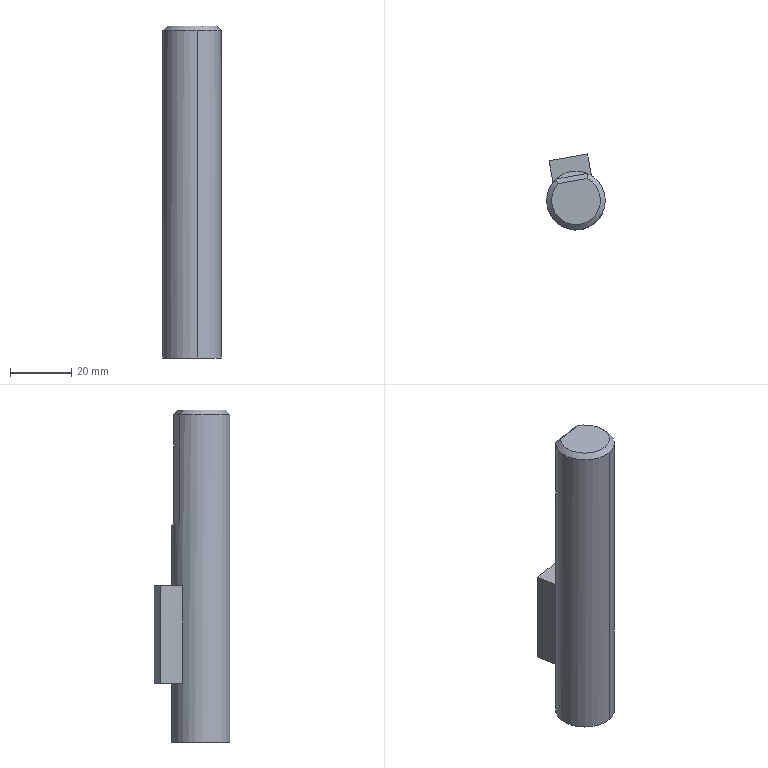Part | SolidWorks | features BaseBody 1 | 1 solid | 13 faces | box 19.2 x 24.894 x 108.8 mm | volume 33278 mm3 | plane 10 | cylinder 2 | cone 1 | commonest cylinder face diameters 19.2 x2
STEP:
#1=CARTESIAN_POINT('',(-315.348,-17.971,516.2));
#2=VERTEX_POINT('',#1);
#3=CARTESIAN_POINT('',(-317.51,-36.226,516.2));
#4=VERTEX_POINT('',#3);
#5=CARTESIAN_POINT('',(-319.181,-26.773,516.2));
#6=DIRECTION('',(0.,0.,-1.));
#7=DIRECTION('',(0.174,-0.9847,0.));
#8=AXIS2_PLACEMENT_3D('',#5,#6,#7);
#9=CIRCLE('',#8,9.6);
#10=EDGE_CURVE('',#2,#4,#9,.T.);
#11=ORIENTED_EDGE('',*,*,#10,.T.);
#12=CARTESIAN_POINT('',(-317.51,-36.226,409.));
#13=VERTEX_POINT('',#12);
#14=CARTESIAN_POINT('',(-317.51,-36.226,460.2));
#15=DIRECTION('',(0.,0.,-1.));
#16=VECTOR('',#15,1000.);
#17=LINE('',#14,#16);
#18=EDGE_CURVE('',#4,#13,#17,.T.);
#19=ORIENTED_EDGE('',*,*,#18,.T.);
#20=CARTESIAN_POINT('',(-320.852,-17.319,409.));
#21=VERTEX_POINT('',#20);
#22=CARTESIAN_POINT('',(-319.181,-26.773,409.));
#23=DIRECTION('',(0.,0.,1.));
#24=DIRECTION('',(0.174,-0.9847,0.));
#25=AXIS2_PLACEMENT_3D('',#22,#23,#24);
#26=CIRCLE('',#25,9.6);
#27=EDGE_CURVE('',#13,#21,#26,.T.);
#28=ORIENTED_EDGE('',*,*,#27,.T.);
#29=CARTESIAN_POINT('',(-320.852,-17.319,428.2));
#30=VERTEX_POINT('',#29);
#31=CARTESIAN_POINT('',(-320.852,-17.319,460.2));
#32=DIRECTION('',(0.,0.,-1.));
#33=VECTOR('',#32,1000.);
#34=LINE('',#31,#33);
#35=EDGE_CURVE('',#30,#21,#34,.T.);
#36=ORIENTED_EDGE('',*,*,#35,.F.);
#37=CARTESIAN_POINT('',(-314.124,-18.613,428.2));
#38=VERTEX_POINT('',#37);
#39=CARTESIAN_POINT('',(-319.181,-26.773,428.2));
#40=DIRECTION('',(0.,0.,-1.));
#41=DIRECTION('',(0.174,-0.9847,0.));
#42=AXIS2_PLACEMENT_3D('',#39,#40,#41);
#43=CIRCLE('',#42,9.6);
#44=EDGE_CURVE('',#30,#38,#43,.T.);
#45=ORIENTED_EDGE('',*,*,#44,.T.);
#46=CARTESIAN_POINT('',(-314.124,-18.613,460.2));
#47=VERTEX_POINT('',#46);
#48=CARTESIAN_POINT('',(-314.124,-18.613,460.2));
#49=DIRECTION('',(0.,0.,-1.));
#50=VECTOR('',#49,1000.);
#51=LINE('',#48,#50);
#52=EDGE_CURVE('',#47,#38,#51,.T.);
#53=ORIENTED_EDGE('',*,*,#52,.F.);
#54=CARTESIAN_POINT('',(-320.852,-17.319,460.2));
#55=VERTEX_POINT('',#54);
#56=CARTESIAN_POINT('',(-319.181,-26.773,460.2));
#57=DIRECTION('',(0.,0.,-1.));
#58=DIRECTION('',(0.174,-0.9847,0.));
#59=AXIS2_PLACEMENT_3D('',#56,#57,#58);
#60=CIRCLE('',#59,9.6);
#61=EDGE_CURVE('',#55,#47,#60,.T.);
#62=ORIENTED_EDGE('',*,*,#61,.F.);
#63=CARTESIAN_POINT('',(-320.852,-17.319,479.4));
#64=VERTEX_POINT('',#63);
#65=CARTESIAN_POINT('',(-320.852,-17.319,460.2));
#66=DIRECTION('',(0.,0.,-1.));
#67=VECTOR('',#66,1000.);
#68=LINE('',#65,#67);
#69=EDGE_CURVE('',#64,#55,#68,.T.);
#70=ORIENTED_EDGE('',*,*,#69,.F.);
#71=CARTESIAN_POINT('',(-315.348,-17.971,481.));
#72=VERTEX_POINT('',#71);
#73=CARTESIAN_POINT('',(-320.852,-17.319,479.4));
#74=CARTESIAN_POINT('',(-318.979,-16.988,479.4));
#75=CARTESIAN_POINT('',(-317.091,-17.212,479.949));
#76=CARTESIAN_POINT('',(-315.348,-17.971,481.));
#77=(BOUNDED_CURVE()B_SPLINE_CURVE(3,(#73,#74,#75,#76),.UNSPECIFIED.,.F.,.F.)B_SPLINE_CURVE_WITH_KNOTS((4,4),(0.,0.5857),.UNSPECIFIED.)CURVE()GEOMETRIC_REPRESENTATION_ITEM()RATIONAL_B_SPLINE_CURVE((1.,0.9716,0.9716,1.))REPRESENTATION_ITEM(''));
#78=EDGE_CURVE('',#64,#72,#77,.T.);
#79=ORIENTED_EDGE('',*,*,#78,.T.);
#80=CARTESIAN_POINT('',(-315.348,-17.971,479.4));
#81=DIRECTION('',(0.,0.,-1.));
#82=VECTOR('',#81,1000.);
#83=LINE('',#80,#82);
#84=EDGE_CURVE('',#2,#72,#83,.T.);
#85=ORIENTED_EDGE('',*,*,#84,.F.);
#86=EDGE_LOOP('',(#11,#19,#28,#36,#45,#53,#62,#70,#79,#85));
#87=FACE_OUTER_BOUND('',#86,.T.);
#88=CARTESIAN_POINT('',(-319.181,-26.773,460.2));
#89=DIRECTION('',(0.,0.,-1.));
#90=DIRECTION('',(-0.174,0.9847,0.));
#91=AXIS2_PLACEMENT_3D('',#88,#89,#90);
#92=CYLINDRICAL_SURFACE('',#91,9.6);
#93=ADVANCED_FACE('',(#87),#92,.T.);
#94=CARTESIAN_POINT('',(-327.989,-13.706,460.2));
#95=VERTEX_POINT('',#94);
#96=CARTESIAN_POINT('',(-326.729,-20.84,460.2));
#97=VERTEX_POINT('',#96);
#98=CARTESIAN_POINT('',(-326.729,-20.84,460.2));
#99=DIRECTION('',(0.174,-0.9847,0.));
#100=VECTOR('',#99,1000.);
#101=LINE('',#98,#100);
#102=EDGE_CURVE('',#95,#97,#101,.T.);
#103=ORIENTED_EDGE('',*,*,#102,.T.);
#104=CARTESIAN_POINT('',(-319.181,-26.773,460.2));
#105=DIRECTION('',(0.,0.,-1.));
#106=DIRECTION('',(0.174,-0.9847,0.));
#107=AXIS2_PLACEMENT_3D('',#104,#105,#106);
#108=CIRCLE('',#107,9.6);
#109=EDGE_CURVE('',#97,#55,#108,.T.);
#110=ORIENTED_EDGE('',*,*,#109,.T.);
#111=ORIENTED_EDGE('',*,*,#61,.T.);
#112=CARTESIAN_POINT('',(-315.385,-11.479,460.2));
#113=VERTEX_POINT('',#112);
#114=CARTESIAN_POINT('',(-314.124,-18.613,460.2));
#115=DIRECTION('',(-0.174,0.9847,0.));
#116=VECTOR('',#115,1000.);
#117=LINE('',#114,#116);
#118=EDGE_CURVE('',#47,#113,#117,.T.);
#119=ORIENTED_EDGE('',*,*,#118,.T.);
#120=CARTESIAN_POINT('',(-327.989,-13.706,460.2));
#121=DIRECTION('',(-0.9847,-0.174,0.));
#122=VECTOR('',#121,1000.);
#123=LINE('',#120,#122);
#124=EDGE_CURVE('',#113,#95,#123,.T.);
#125=ORIENTED_EDGE('',*,*,#124,.T.);
#126=EDGE_LOOP('',(#103,#110,#111,#119,#125));
#127=FACE_OUTER_BOUND('',#126,.T.);
#128=CARTESIAN_POINT('',(-319.181,-26.773,460.2));
#129=DIRECTION('',(0.,0.,1.));
#130=DIRECTION('',(0.174,-0.9847,0.));
#131=AXIS2_PLACEMENT_3D('',#128,#129,#130);
#132=PLANE('',#131);
#133=ADVANCED_FACE('',(#127),#132,.T.);
#134=CARTESIAN_POINT('',(-326.729,-20.84,428.2));
#135=VERTEX_POINT('',#134);
#136=CARTESIAN_POINT('',(-319.181,-26.773,428.2));
#137=DIRECTION('',(0.,0.,-1.));
#138=DIRECTION('',(0.174,-0.9847,0.));
#139=AXIS2_PLACEMENT_3D('',#136,#137,#138);
#140=CIRCLE('',#139,9.6);
#141=EDGE_CURVE('',#135,#30,#140,.T.);
#142=ORIENTED_EDGE('',*,*,#141,.F.);
#143=CARTESIAN_POINT('',(-327.989,-13.706,428.2));
#144=VERTEX_POINT('',#143);
#145=CARTESIAN_POINT('',(-326.729,-20.84,428.2));
#146=DIRECTION('',(0.174,-0.9847,0.));
#147=VECTOR('',#146,1000.);
#148=LINE('',#145,#147);
#149=EDGE_CURVE('',#144,#135,#148,.T.);
#150=ORIENTED_EDGE('',*,*,#149,.F.);
#151=CARTESIAN_POINT('',(-315.385,-11.479,428.2));
#152=VERTEX_POINT('',#151);
#153=CARTESIAN_POINT('',(-327.989,-13.706,428.2));
#154=DIRECTION('',(-0.9847,-0.174,0.));
#155=VECTOR('',#154,1000.);
#156=LINE('',#153,#155);
#157=EDGE_CURVE('',#152,#144,#156,.T.);
#158=ORIENTED_EDGE('',*,*,#157,.F.);
#159=CARTESIAN_POINT('',(-314.124,-18.613,428.2));
#160=DIRECTION('',(-0.174,0.9847,0.));
#161=VECTOR('',#160,1000.);
#162=LINE('',#159,#161);
#163=EDGE_CURVE('',#38,#152,#162,.T.);
#164=ORIENTED_EDGE('',*,*,#163,.F.);
#165=ORIENTED_EDGE('',*,*,#44,.F.);
#166=EDGE_LOOP('',(#142,#150,#158,#164,#165));
#167=FACE_OUTER_BOUND('',#166,.T.);
#168=CARTESIAN_POINT('',(-319.181,-26.773,428.2));
#169=DIRECTION('',(0.,0.,1.));
#170=DIRECTION('',(0.174,-0.9847,0.));
#171=AXIS2_PLACEMENT_3D('',#168,#169,#170);
#172=PLANE('',#171);
#173=ADVANCED_FACE('',(#167),#172,.F.);
#174=ORIENTED_EDGE('',*,*,#157,.T.);
#175=CARTESIAN_POINT('',(-327.989,-13.706,460.2));
#176=DIRECTION('',(0.,0.,-1.));
#177=VECTOR('',#176,1000.);
#178=LINE('',#175,#177);
#179=EDGE_CURVE('',#95,#144,#178,.T.);
#180=ORIENTED_EDGE('',*,*,#179,.F.);
#181=ORIENTED_EDGE('',*,*,#124,.F.);
#182=CARTESIAN_POINT('',(-315.385,-11.479,460.2));
#183=DIRECTION('',(0.,0.,-1.));
#184=VECTOR('',#183,1000.);
#185=LINE('',#182,#184);
#186=EDGE_CURVE('',#113,#152,#185,.T.);
#187=ORIENTED_EDGE('',*,*,#186,.T.);
#188=EDGE_LOOP('',(#174,#180,#181,#187));
#189=FACE_OUTER_BOUND('',#188,.T.);
#190=CARTESIAN_POINT('',(-327.989,-13.706,460.2));
#191=DIRECTION('',(0.174,-0.9847,0.));
#192=DIRECTION('',(0.9847,0.174,0.));
#193=AXIS2_PLACEMENT_3D('',#190,#191,#192);
#194=PLANE('',#193);
#195=ADVANCED_FACE('',(#189),#194,.F.);
#196=ORIENTED_EDGE('',*,*,#149,.T.);
#197=CARTESIAN_POINT('',(-326.729,-20.84,460.2));
#198=DIRECTION('',(0.,0.,-1.));
#199=VECTOR('',#198,1000.);
#200=LINE('',#197,#199);
#201=EDGE_CURVE('',#97,#135,#200,.T.);
#202=ORIENTED_EDGE('',*,*,#201,.F.);
#203=ORIENTED_EDGE('',*,*,#102,.F.);
#204=ORIENTED_EDGE('',*,*,#179,.T.);
#205=EDGE_LOOP('',(#196,#202,#203,#204));
#206=FACE_OUTER_BOUND('',#205,.T.);
#207=CARTESIAN_POINT('',(-326.729,-20.84,460.2));
#208=DIRECTION('',(0.9847,0.174,0.));
#209=DIRECTION('',(-0.174,0.9847,0.));
#210=AXIS2_PLACEMENT_3D('',#207,#208,#209);
#211=PLANE('',#210);
#212=ADVANCED_FACE('',(#206),#211,.F.);
#213=ORIENTED_EDGE('',*,*,#18,.F.);
#214=CARTESIAN_POINT('',(-325.799,-19.818,516.2));
#215=VERTEX_POINT('',#214);
#216=CARTESIAN_POINT('',(-319.181,-26.773,516.2));
#217=DIRECTION('',(0.,0.,-1.));
#218=DIRECTION('',(0.174,-0.9847,0.));
#219=AXIS2_PLACEMENT_3D('',#216,#217,#218);
#220=CIRCLE('',#219,9.6);
#221=EDGE_CURVE('',#4,#215,#220,.T.);
#222=ORIENTED_EDGE('',*,*,#221,.T.);
#223=CARTESIAN_POINT('',(-325.799,-19.818,481.));
#224=VERTEX_POINT('',#223);
#225=CARTESIAN_POINT('',(-325.799,-19.818,479.4));
#226=DIRECTION('',(0.,0.,-1.));
#227=VECTOR('',#226,1000.);
#228=LINE('',#225,#227);
#229=EDGE_CURVE('',#215,#224,#228,.T.);
#230=ORIENTED_EDGE('',*,*,#229,.T.);
#231=CARTESIAN_POINT('',(-325.799,-19.818,481.));
#232=CARTESIAN_POINT('',(-324.421,-18.507,479.949));
#233=CARTESIAN_POINT('',(-322.724,-17.65,479.4));
#234=CARTESIAN_POINT('',(-320.852,-17.319,479.4));
#235=(BOUNDED_CURVE()B_SPLINE_CURVE(3,(#231,#232,#233,#234),.UNSPECIFIED.,.F.,.F.)B_SPLINE_CURVE_WITH_KNOTS((4,4),(5.697,6.283),.UNSPECIFIED.)CURVE()GEOMETRIC_REPRESENTATION_ITEM()RATIONAL_B_SPLINE_CURVE((1.,0.9716,0.9716,1.))REPRESENTATION_ITEM(''));
#236=EDGE_CURVE('',#224,#64,#235,.T.);
#237=ORIENTED_EDGE('',*,*,#236,.T.);
#238=ORIENTED_EDGE('',*,*,#69,.T.);
#239=ORIENTED_EDGE('',*,*,#109,.F.);
#240=ORIENTED_EDGE('',*,*,#201,.T.);
#241=ORIENTED_EDGE('',*,*,#141,.T.);
#242=ORIENTED_EDGE('',*,*,#35,.T.);
#243=CARTESIAN_POINT('',(-319.181,-26.773,409.));
#244=DIRECTION('',(0.,0.,1.));
#245=DIRECTION('',(0.174,-0.9847,0.));
#246=AXIS2_PLACEMENT_3D('',#243,#244,#245);
#247=CIRCLE('',#246,9.6);
#248=EDGE_CURVE('',#21,#13,#247,.T.);
#249=ORIENTED_EDGE('',*,*,#248,.T.);
#250=EDGE_LOOP('',(#213,#222,#230,#237,#238,#239,#240,#241,#242,#249));
#251=FACE_OUTER_BOUND('',#250,.T.);
#252=CARTESIAN_POINT('',(-319.181,-26.773,460.2));
#253=DIRECTION('',(0.,0.,-1.));
#254=DIRECTION('',(-0.174,0.9847,0.));
#255=AXIS2_PLACEMENT_3D('',#252,#253,#254);
#256=CYLINDRICAL_SURFACE('',#255,9.6);
#257=ADVANCED_FACE('',(#251),#256,.T.);
#258=ORIENTED_EDGE('',*,*,#163,.T.);
#259=ORIENTED_EDGE('',*,*,#186,.F.);
#260=ORIENTED_EDGE('',*,*,#118,.F.);
#261=ORIENTED_EDGE('',*,*,#52,.T.);
#262=EDGE_LOOP('',(#258,#259,#260,#261));
#263=FACE_OUTER_BOUND('',#262,.T.);
#264=CARTESIAN_POINT('',(-314.124,-18.613,460.2));
#265=DIRECTION('',(-0.9847,-0.174,0.));
#266=DIRECTION('',(0.174,-0.9847,0.));
#267=AXIS2_PLACEMENT_3D('',#264,#265,#266);
#268=PLANE('',#267);
#269=ADVANCED_FACE('',(#263),#268,.F.);
#270=ORIENTED_EDGE('',*,*,#248,.F.);
#271=ORIENTED_EDGE('',*,*,#27,.F.);
#272=EDGE_LOOP('',(#270,#271));
#273=FACE_OUTER_BOUND('',#272,.T.);
#274=CARTESIAN_POINT('',(-319.181,-26.773,409.));
#275=DIRECTION('',(0.,0.,1.));
#276=DIRECTION('',(0.174,-0.9847,0.));
#277=AXIS2_PLACEMENT_3D('',#274,#275,#276);
#278=PLANE('',#277);
#279=ADVANCED_FACE('',(#273),#278,.F.);
#280=CARTESIAN_POINT('',(-315.568,-19.635,517.8));
#281=VERTEX_POINT('',#280);
#282=CARTESIAN_POINT('',(-325.022,-21.306,517.8));
#283=VERTEX_POINT('',#282);
#284=CARTESIAN_POINT('',(-325.52,-21.394,517.8));
#285=DIRECTION('',(-0.9847,-0.174,0.));
#286=VECTOR('',#285,1000.);
#287=LINE('',#284,#286);
#288=EDGE_CURVE('',#281,#283,#287,.T.);
#289=ORIENTED_EDGE('',*,*,#288,.T.);
#290=CARTESIAN_POINT('',(-319.181,-26.773,517.8));
#291=DIRECTION('',(0.,0.,1.));
#292=DIRECTION('',(0.174,-0.9847,0.));
#293=AXIS2_PLACEMENT_3D('',#290,#291,#292);
#294=CIRCLE('',#293,8.);
#295=EDGE_CURVE('',#283,#281,#294,.T.);
#296=ORIENTED_EDGE('',*,*,#295,.T.);
#297=EDGE_LOOP('',(#289,#296));
#298=FACE_OUTER_BOUND('',#297,.T.);
#299=CARTESIAN_POINT('',(-319.181,-26.773,517.8));
#300=DIRECTION('',(0.,0.,1.));
#301=DIRECTION('',(0.174,-0.9847,0.));
#302=AXIS2_PLACEMENT_3D('',#299,#300,#301);
#303=PLANE('',#302);
#304=ADVANCED_FACE('',(#298),#303,.T.);
#305=ORIENTED_EDGE('',*,*,#229,.F.);
#306=CARTESIAN_POINT('',(-315.348,-17.971,516.2));
#307=DIRECTION('',(0.9847,0.174,0.));
#308=VECTOR('',#307,1000.);
#309=LINE('',#306,#308);
#310=EDGE_CURVE('',#215,#2,#309,.T.);
#311=ORIENTED_EDGE('',*,*,#310,.T.);
#312=ORIENTED_EDGE('',*,*,#84,.T.);
#313=CARTESIAN_POINT('',(-325.799,-19.818,481.));
#314=DIRECTION('',(-0.9847,-0.174,0.));
#315=VECTOR('',#314,1000.);
#316=LINE('',#313,#315);
#317=EDGE_CURVE('',#72,#224,#316,.T.);
#318=ORIENTED_EDGE('',*,*,#317,.T.);
#319=EDGE_LOOP('',(#305,#311,#312,#318));
#320=FACE_OUTER_BOUND('',#319,.T.);
#321=CARTESIAN_POINT('',(-325.799,-19.818,479.4));
#322=DIRECTION('',(0.174,-0.9847,0.));
#323=DIRECTION('',(0.9847,0.174,0.));
#324=AXIS2_PLACEMENT_3D('',#321,#322,#323);
#325=PLANE('',#324);
#326=ADVANCED_FACE('',(#320),#325,.F.);
#327=CARTESIAN_POINT('',(-315.348,-17.971,516.2));
#328=CARTESIAN_POINT('',(-315.413,-18.526,516.735));
#329=CARTESIAN_POINT('',(-315.486,-19.08,517.268));
#330=CARTESIAN_POINT('',(-315.568,-19.635,517.8));
#331=B_SPLINE_CURVE_WITH_KNOTS('',3,(#327,#328,#329,#330),.UNSPECIFIED.,.F.,.F.,(4,4),(0.,0.002319),.UNSPECIFIED.);
#332=EDGE_CURVE('',#2,#281,#331,.T.);
#333=ORIENTED_EDGE('',*,*,#332,.F.);
#334=ORIENTED_EDGE('',*,*,#310,.F.);
#335=CARTESIAN_POINT('',(-325.022,-21.306,517.8));
#336=CARTESIAN_POINT('',(-325.289,-20.813,517.268));
#337=CARTESIAN_POINT('',(-325.547,-20.316,516.735));
#338=CARTESIAN_POINT('',(-325.799,-19.818,516.2));
#339=B_SPLINE_CURVE_WITH_KNOTS('',3,(#335,#336,#337,#338),.UNSPECIFIED.,.F.,.F.,(4,4),(0.,0.002319),.UNSPECIFIED.);
#340=EDGE_CURVE('',#283,#215,#339,.T.);
#341=ORIENTED_EDGE('',*,*,#340,.F.);
#342=ORIENTED_EDGE('',*,*,#288,.F.);
#343=EDGE_LOOP('',(#333,#334,#341,#342));
#344=FACE_OUTER_BOUND('',#343,.T.);
#345=CARTESIAN_POINT('',(-325.799,-19.818,516.2));
#346=DIRECTION('',(-0.1231,0.6963,0.7071));
#347=DIRECTION('',(-0.9847,-0.174,0.));
#348=AXIS2_PLACEMENT_3D('',#345,#346,#347);
#349=PLANE('',#348);
#350=ADVANCED_FACE('',(#344),#349,.T.);
#351=ORIENTED_EDGE('',*,*,#340,.T.);
#352=ORIENTED_EDGE('',*,*,#221,.F.);
#353=ORIENTED_EDGE('',*,*,#10,.F.);
#354=ORIENTED_EDGE('',*,*,#332,.T.);
#355=ORIENTED_EDGE('',*,*,#295,.F.);
#356=EDGE_LOOP('',(#351,#352,#353,#354,#355));
#357=FACE_OUTER_BOUND('',#356,.T.);
#358=CARTESIAN_POINT('',(-319.181,-26.773,517.8));
#359=DIRECTION('',(0.,0.,-1.));
#360=DIRECTION('',(-0.174,0.9847,0.));
#361=AXIS2_PLACEMENT_3D('',#358,#359,#360);
#362=CONICAL_SURFACE('',#361,8.,0.7854);
#363=ADVANCED_FACE('',(#357),#362,.T.);
#364=ORIENTED_EDGE('',*,*,#236,.F.);
#365=ORIENTED_EDGE('',*,*,#317,.F.);
#366=ORIENTED_EDGE('',*,*,#78,.F.);
#367=EDGE_LOOP('',(#364,#365,#366));
#368=FACE_OUTER_BOUND('',#367,.T.);
#369=CARTESIAN_POINT('',(-320.852,-17.319,479.4));
#370=DIRECTION('',(0.1231,-0.6963,-0.7071));
#371=DIRECTION('',(0.9847,0.174,0.));
#372=AXIS2_PLACEMENT_3D('',#369,#370,#371);
#373=PLANE('',#372);
#374=ADVANCED_FACE('',(#368),#373,.F.);
#375=CLOSED_SHELL('',(#93,#133,#173,#195,#212,#257,#269,#279,#304,#326,#350,#363,#374));
#376=MANIFOLD_SOLID_BREP('',#375);
#377=CARTESIAN_POINT('',(0.,0.,0.));
#378=DIRECTION('',(0.,0.,1.));
#379=DIRECTION('',(1.,0.,0.));
#380=AXIS2_PLACEMENT_3D('',#377,#378,#379);
#381=(LENGTH_UNIT()NAMED_UNIT(*)SI_UNIT(.MILLI.,.METRE.));
#382=UNCERTAINTY_MEASURE_WITH_UNIT(LENGTH_MEASURE(0.00001),#381,'','');
#383=(NAMED_UNIT(*)PLANE_ANGLE_UNIT()SI_UNIT($,.RADIAN.));
#384=(NAMED_UNIT(*)SI_UNIT($,.STERADIAN.)SOLID_ANGLE_UNIT());
#385=(GEOMETRIC_REPRESENTATION_CONTEXT(3)GLOBAL_UNCERTAINTY_ASSIGNED_CONTEXT((#382))GLOBAL_UNIT_ASSIGNED_CONTEXT((#381,#383,#384))REPRESENTATION_CONTEXT('',''));
#386=ADVANCED_BREP_SHAPE_REPRESENTATION('',(#376,#380),#385);